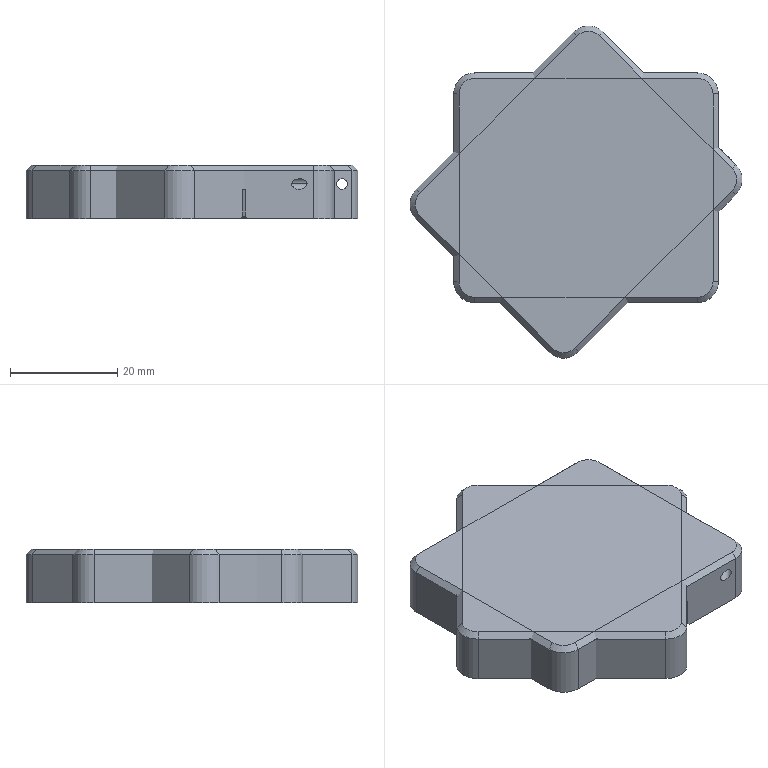NC program | NX | posted with a generic post | part box 61.954 x 61.954 x 10 mm
Whole program:
N10 G17 G21 G94 G90
(ADAPTIVE_MILLING_1 , TOOL : D12开粗)
N12 T02 M6
N14 G54
N16 G17 G0 G90 X-47.087 Y-3.5 B0. C0. S5500 M3
N18 G43 Z30. H2
N20 Z3.1
N22 G94 G1 X-46.937 Y-3.498 Z2.163 F3000.
N24 X-46.787 Y-3.495 Z1.792
N26 X-46.637 Y-3.493 Z1.52
N28 X-46.487 Y-3.491 Z1.3
N30 X-46.337 Y-3.489 Z1.116
N32 X-46.187 Y-3.486 Z0.958
N34 X-46.037 Y-3.484 Z0.82
N36 X-45.887 Y-3.482 Z0.7
N38 X-45.737 Y-3.48 Z0.595
N40 X-45.587 Y-3.477 Z0.502
N42 X-45.437 Y-3.475 Z0.421
N44 X-45.287 Y-3.473 Z0.35
N46 X-45.137 Y-3.471 Z0.29
N48 X-44.987 Y-3.468 Z0.238
N50 X-44.837 Y-3.466 Z0.195
N52 X-44.687 Y-3.464 Z0.161
N54 X-44.537 Y-3.461 Z0.134
N56 X-44.387 Y-3.459 Z0.115
N58 X-44.237 Y-3.457 Z0.104
N60 X-44.087 Y-3.455 Z0.1
N62 X-42.192 Y-3.426
N64 G3 X-41.079 Y-2.649 R1.212
N66 X-40.463 Y0.387 R10.505
N68 X-40.211 Y9.098 R113.687
N70 G1 X-40.2 Y15.678
N72 G2 X-40.18 Y25.077 R512.012
N74 X-37.742 Y29.525 R6.753
N76 X-32.923 Y31.847 R11.427
N78 X-26.975 Y32.564 R31.338
N80 X-14.377 Y32.697 R338.946
N82 G1 X32.076 Y32.698
N84 G2 X36.615 Y30.681 R6.437
N86 X39.166 Y26.099 R10.567
N88 X40.03 Y20.175 R26.789
N90 X40.197 Y9.077 R234.041
N92 G1 X40.199 Y4.677
N94 X40.198 Y-24.619
N96 G2 X38.149 Y-29.145 R6.461
N98 X33.459 Y-31.704 R10.679
N100 X27.429 Y-32.542 R27.958
N102 X16.631 Y-32.696 R246.645
N104 G1 X12.231 Y-32.698
N106 X-32.12 Y-32.697
N108 G2 X-36.646 Y-30.648 R6.462
N110 X-39.205 Y-25.958 R10.681
N112 X-40.042 Y-19.928 R27.995
N114 X-40.196 Y-9.63 R235.867
N116 X-40.144 Y-4.832 R77.851
N118 G3 X-39.603 Y1.94 R216.935
N120 X-39.403 Y14.082 R271.781
N122 G2 X-39.382 Y22.177 R675.391
N124 X-35.797 Y28.613 R8.725
N126 X-30.23 Y31.026 R14.206
N128 X-23.379 Y31.77 R39.402
N130 X-8.58 Y31.898 R456.141
N132 G1 X29.375 Y31.894
N134 G2 X36.05 Y28.379 R8.688
N136 X38.481 Y22.929 R13.975
N138 X39.258 Y16.183 R37.505
N140 X39.397 Y3.784 R341.277
N142 G1 X39.399 Y-21.673
N144 G2 X35.879 Y-28.547 R8.684
N146 X30.331 Y-31.002 R14.053
N148 X23.383 Y-31.769 R38.852
N150 X8.684 Y-31.898 R449.577
N152 G1 X-29.374 Y-31.894
N154 G2 X-36.048 Y-28.378 R8.693
N156 X-38.503 Y-22.828 R14.057
N158 X-39.27 Y-15.88 R38.87
N160 X-39.332 Y-6.182 R142.573
N162 G1 X-38.853 Y1.436
N164 G3 X-38.603 Y15.882 R310.927
N166 G2 X-38.55 Y20.277 R69.413
N168 X-33.953 Y27.909 R10.066
N170 X-27.936 Y30.252 R16.526
N172 X-20.479 Y30.979 R47.05
N174 X-4.98 Y31.097 R535.572
N176 G1 X26.676 Y31.095
N178 G2 X35.514 Y26.29 R10.159
N180 X37.751 Y20.441 R16.681
N182 X38.476 Y13.085 R46.537
N184 X38.598 Y-1.914 R501.258
N186 G1 X38.596 Y-19.214
N188 G2 X33.768 Y-28.028 R10.153
N190 X27.712 Y-30.295 R16.914
N192 X19.952 Y-30.995 R50.455
N194 X4.952 Y-31.097 R603.511
N196 G1 X-26.648 Y-31.095
N198 G2 X-35.516 Y-26.283 R10.16
N200 X-37.795 Y-20.212 R16.896
N202 X-38.486 Y-12.752 R49.142
N204 X-38.238 Y-1.822 R104.868
N206 G3 X-37.806 Y15.587 R293.259
N208 G2 X-37.576 Y19.674 R22.707
N210 X-32.426 Y27.107 R11.028
N212 X-26.079 Y29.448 R18.166
N214 X-18.02 Y30.185 R52.988
N216 X-3.321 Y30.297 R554.733
N218 G1 X24.176 Y30.296
N220 G2 X29.09 Y29.547 R13.62
N222 X34.915 Y24.413 R11.35
N224 X37.037 Y18.092 R19.251
N226 X37.706 Y9.826 R58.88
N228 X37.798 Y-4.474 R658.765
N230 G1 X37.797 Y-16.673
N232 G2 X37.048 Y-21.588 R13.63
N234 X31.911 Y-27.415 R11.354
N236 X25.587 Y-29.536 R19.254
N238 X17.321 Y-30.205 R59.081
N240 X2.722 Y-30.297 R679.393
N242 G1 X-24.374 Y-30.295
N244 G2 X-29.46 Y-29.398 R12.958
N246 X-35.108 Y-24.06 R11.555
N248 X-37.117 Y-17.592 R20.289
N250 X-37.639 Y-6.819 R60.735
N252 X-37.245 Y2.173 R815.993
N254 G3 X-36.996 Y15.605 R483.083
N256 G2 X-35.771 Y21.228 R13.51
N258 X-30.172 Y26.781 R12.359
N260 X-23.494 Y28.798 R21.693
N262 X-14.822 Y29.416 R68.888
N264 X-0.423 Y29.496 R791.053
N266 G1 X22.175 Y29.495
N268 G2 X27.024 Y28.921 R16.905
N270 X33.89 Y23.379 R11.863
N272 X36.148 Y16.887 R19.749
N274 X36.888 Y8.427 R57.67
N276 X36.997 Y-6.572 R593.977
N278 X36.968 Y-15.973 R491.337
N280 X35.306 Y-22.082 R12.637
N282 X29.546 Y-27.084 R12.801
N284 X22.803 Y-28.895 R23.527
N286 X13.724 Y-29.437 R80.469
N288 X0.524 Y-29.496 R796.232
N290 G1 X-22.174 Y-29.495
N292 G2 X-27.022 Y-28.92 R16.896
N294 X-33.889 Y-23.375 R11.869
N296 X-36.129 Y-16.98 R19.668
N298 X-36.788 Y-7.517 R49.35
N300 X-36.414 Y3.241 R588.04
N302 G3 X-36.194 Y14.226 R985.921
N304 G2 X-34.978 Y19.858 R14.612
N306 X-29.08 Y25.845 R12.846
N308 X-22.127 Y27.962 R22.483
N310 X-13.057 Y28.613 R71.08
N312 X1.843 Y28.696 R805.214
N314 G1 X20.176 Y28.695
N316 G2 X25.142 Y28.232 R21.058
N318 X32.876 Y22.413 R12.364
N320 X35.285 Y15.664 R20.243
N322 X36.074 Y7.008 R57.951
N324 X36.196 Y-8.391 R556.749
N326 X36.14 Y-14.773 R145.792
N328 X34.231 Y-21.221 R13.268
N330 X28.224 Y-26.257 R13.497
N332 X21.186 Y-28.094 R24.935
N334 X12.006 Y-28.634 R84.46
N336 X-1.194 Y-28.696 R789.14
N338 G1 X-20.194 Y-28.694
N340 G2 X-25.159 Y-28.226 R20.841
N342 X-32.953 Y-22.279 R12.39
N344 X-35.304 Y-15.514 R20.401
N346 X-35.907 Y-6.747 R48.303
N348 X-35.566 Y5.105 R774.796
N350 X-35.388 Y13.046 R564.731
N352 X-34.008 Y18.946 R15.215
N354 X-27.932 Y24.979 R13.372
N356 X-20.98 Y27.108 R23.087
N358 X-12.313 Y27.788 R67.73
N360 X2.586 Y27.895 R629.437
N362 G1 X18.386 Y27.894
N364 G2 X23.559 Y27.471 R24.709
N366 X32.07 Y21.168 R12.879
N368 X34.447 Y14.4 R21.12
N370 X35.263 Y5.646 R58.782
N372 X35.359 Y-12.752 R477.337
N374 X34.193 Y-18.5 R15.721
N376 X28.182 Y-24.841 R13.195
N378 X21.148 Y-27.078 R22.584
N380 X12.483 Y-27.782 R65.83
N382 X-3.516 Y-27.895 R642.924
N384 G1 X-18.274 Y-27.894
N386 G2 X-23.449 Y-27.493 R25.544
N388 X-32.068 Y-21.165 R12.877
N390 X-34.476 Y-14.09 R20.871
N392 X-35.029 Y-5.619 R50.258
N394 X-34.752 Y5.89 R768.444
N396 X-34.567 Y12.167 R144.064
N398 X-32.826 Y18.484 R15.184
N400 X-26.471 Y24.296 R14.08
N402 X-19.385 Y26.337 R24.783
N404 X-9.915 Y27.007 R76.762
N406 X4.484 Y27.095 R780.18
N408 G1 X16.876 Y27.092
N410 G2 X22.249 Y26.663 R26.883
N412 X31.171 Y20.134 R13.309
N414 X33.634 Y13.085 R21.832
N416 X34.459 Y4.132 R61.158
N418 X34.554 Y-11.267 R352.152
N420 X33.479 Y-17.038 R17.132
N422 X27.197 Y-23.916 R13.523
N424 X20.09 Y-26.22 R22.917
N426 X11.129 Y-26.974 R65.955
N428 X-4.57 Y-27.095 R601.629
N430 G1 X-16.57 Y-27.094
N432 G2 X-21.949 Y-26.721 R29.489
N434 X-31.269 Y-19.954 R13.341
N436 X-33.631 Y-12.771 R21.45
N438 X-34.159 Y-4.297 R53.449
N440 X-33.827 Y10.181 R613.148
N442 X-32.604 Y16.126 R17.909
N444 X-26.094 Y23.091 R14.015
N446 X-18.886 Y25.402 R23.656
N448 X-9.925 Y26.164 R66.715
N450 X6.574 Y26.295 R603.817
N452 X17.273 Y26.255 R504.016
N454 X23.066 Y25.276 R18.786
N456 X30.475 Y18.785 R13.831
N458 X32.862 Y11.605 R23.098
N460 X33.661 Y2.548 R64.779
N462 X33.74 Y-10.05 R239.906
N464 X32.642 Y-15.919 R17.856
N466 X26.098 Y-23.074 R13.914
N468 X18.987 Y-25.38 R23.444
N470 X9.829 Y-26.166 R66.354
N472 X-6.27 Y-26.294 R597.162
N474 X-17.174 Y-26.258 R495.505
N476 X-22.878 Y-25.341 R19.251
N478 X-30.457 Y-18.789 R13.736
N480 X-32.752 Y-11.68 R21.853
N482 X-33.297 Y-3.106 R55.449
N484 X-33.039 Y8.983 R305.003
N486 X-31.792 Y15.027 R18.742
N488 X-25.173 Y22.181 R14.328
N490 X-17.978 Y24.537 R23.837
N492 X-8.722 Y25.356 R66.184
N494 X8.077 Y25.494 R588.727
N496 X16.575 Y25.423 R209.725
N498 X22.62 Y24.194 R17.974
N500 X29.679 Y17.644 R14.244
N502 X32.04 Y10.447 R23.786
N504 X32.851 Y1.391 R65.28
N506 X32.916 Y-9.007 R159.97
N508 X31.678 Y-15.151 R17.919
N510 X25.19 Y-22.151 R14.244
N512 X17.996 Y-24.528 R23.665
N514 X8.741 Y-25.354 R65.627
N516 X-8.458 Y-25.494 R598.535
N518 X-16.656 Y-25.417 R186.832
N520 X-22.787 Y-24.121 R17.683
N522 X-29.797 Y-17.358 R14.191
N524 X-31.968 Y-10. R23.332
N526 X-32.444 Y-1.02 R64.421
N528 X-32.217 Y8.275 R151.413
N530 X-30.718 Y14.564 R18.12
N532 X-23.961 Y21.44 R14.781
N534 X-16.547 Y23.771 R24.934
N536 X-7.187 Y24.56 R70.271
N538 X14.412 Y24.655 R644.798
N540 X20.236 Y23.836 R22.251
N542 X28.703 Y16.862 R14.396
N544 X31.152 Y9.695 R23.603
N546 X32.038 Y0.345 R63.647
N548 X32.076 Y-8.153 R104.784
N550 X30.683 Y-14.464 R17.671
N552 X24.029 Y-21.379 R14.587
N554 X16.632 Y-23.75 R24.626
N556 X7.474 Y-24.549 R68.103
N558 X-9.824 Y-24.694 R591.965
N560 X-16.42 Y-24.539 R79.28
N562 X-23.184 Y-22.567 R16.171
N564 X-29.199 Y-15.781 R14.816
N566 X-31.199 Y-8.17 R25.383
N568 X-31.597 Y1.115 R76.181
N570 X-31.327 Y8.107 R68.591
N572 X-29.12 Y15.002 R16.536
N574 X-22.425 Y20.868 R15.514
N576 X-14.961 Y23.033 R26.857
N578 X-5.395 Y23.773 R77.026
N580 X13.403 Y23.844 R484.321
N582 X19.416 Y22.938 R22.243
N584 X27.784 Y15.998 R14.649
N586 X30.343 Y8.546 R23.972
N588 X31.223 Y-0.603 R63.698
N590 X31.173 Y-7.998 R61.479
N592 X29.024 Y-15.012 R16.112
N594 X22.44 Y-20.832 R15.346
N596 X14.78 Y-23.054 R26.829
N598 X5.513 Y-23.768 R76.96
N600 X-13.286 Y-23.847 R498.573
N602 X-19.304 Y-22.971 R22.656
N604 X-27.851 Y-15.751 R14.455
N606 X-30.182 Y-8.241 R23.424
N608 X-30.754 Y1.033 R64.446
N610 X-30.418 Y7.819 R47.863
N612 X-27.144 Y15.654 R15.701
N614 X-20.173 Y20.583 R16.838
N616 X-12.404 Y22.425 R31.622
N618 X-2.026 Y23.02 R102.326
N620 X12.073 Y23.044 R402.694
N622 X18.289 Y22.145 R23.455
N624 X26.968 Y14.975 R14.921
N626 X29.5 Y7.612 R24.319
N628 X30.424 Y-2.235 R63.43
N630 X30.098 Y-8.716 R33.378
N632 X22.511 Y-19.438 R14.847
N634 X15.064 Y-22.004 R24.247
N636 X5.617 Y-22.921 R64.543
N638 X-12.08 Y-23.043 R382.648
N640 X-18.104 Y-22.198 R23.668
N642 X-27.036 Y-14.675 R14.682
N644 X-29.316 Y-7.248 R23.973
N646 X-29.723 Y5.719 R59.734
N648 X-27.637 Y12.761 R17.448
N650 X-20.718 Y19.078 R15.811
N652 X-12.983 Y21.379 R27.22
N654 X-3.321 Y22.157 R76.946
N656 X11.278 Y22.224 R281.36
N658 X17.483 Y21.257 R22.963
N660 X26.132 Y14.007 R15.16
N662 X28.684 Y6.564 R24.744
N664 X29.49 Y-5.583 R52.906
N666 X27.553 Y-12.668 R16.907
N668 X20.753 Y-19.018 R15.545
N670 X13.32 Y-21.312 R26.419
N672 X3.562 Y-22.148 R72.859
N674 X-11.336 Y-22.222 R276.001
N676 X-17.632 Y-21.203 R22.555
N678 X-26.136 Y-13.777 R14.883
N680 X-28.456 Y-6.254 R24.259
N682 X-28.847 Y5.013 R47.774
N684 X-26.465 Y12.374 R16.949
N686 X-19.499 Y18.372 R16.218
N688 X-11.735 Y20.6 R28.291
N690 X-1.97 Y21.361 R80.32
N692 X10.328 Y21.409 R211.35
N694 X16.72 Y20.359 R22.889
N696 X25.336 Y12.982 R15.405
N698 X27.905 Y5.336 R25.378
N700 X28.579 Y-4.917 R42.719
N702 X26.235 Y-12.493 R16.284
N704 X19.541 Y-18.303 R15.96
N706 X11.881 Y-20.564 R27.576
N708 X2.02 Y-21.357 R77.747
N710 X-10.378 Y-21.406 R207.67
N712 X-16.576 Y-20.399 R22.758
N714 X-25.247 Y-12.876 R15.038
N716 X-27.601 Y-5.264 R24.573
N718 X-27.938 Y4.405 R38.333
N720 X-25.047 Y12.297 R16.335
N722 X-18.032 Y17.777 R16.826
N724 X-10.127 Y19.874 R30.253
N726 X0.243 Y20.587 R90.867
N728 X9.94 Y20.562 R132.849
N730 X16.488 Y19.265 R21.092
N732 X24.554 Y11.947 R15.64
N734 X27.096 Y4.279 R25.737
N736 X27.623 Y-4.482 R34.143
N738 X24.505 Y-12.792 R15.538
N740 X17.664 Y-17.887 R16.874
N742 X9.739 Y-19.917 R30.909
N744 X-0.334 Y-20.587 R93.156
N746 X-9.732 Y-20.573 R137.837
N748 X-16.193 Y-19.363 R21.519
N750 X-24.319 Y-12.062 R15.191
N752 X-26.75 Y-4.243 R24.619
N754 X-26.917 Y4.426 R30.072
N756 X-18.905 Y16.044 R15.566
N758 X-11.286 Y18.699 R25.3
N760 X-1.644 Y19.688 R65.027
N762 X8.952 Y19.742 R119.084
N764 X15.499 Y18.455 R21.447
N766 X23.686 Y11.085 R15.801
N768 X26.295 Y3.121 R25.587
N770 X26.561 Y-4.646 R26.347
N772 X19.195 Y-15.789 R15.063
N774 X11.627 Y-18.609 R24.089
N776 X2.195 Y-19.659 R60.494
N778 X-8.901 Y-19.744 R121.022
N780 X-15.353 Y-18.489 R21.289
N782 X-23.47 Y-11.112 R15.361
N784 X-25.952 Y-2.716 R24.58
N786 X-25.753 Y4.847 R22.965
N788 X-18.365 Y14.985 R15.375
N790 X-10.799 Y17.785 R24.533
N792 X-1.369 Y18.848 R60.637
N794 X8.127 Y18.907 R94.394
N796 X14.76 Y17.549 R21.147
N798 X22.88 Y10.117 R15.979
N800 X25.641 Y-3.237 R25.057
N802 X18.527 Y-14.78 R14.926
N804 X11.103 Y-17.692 R23.421
N806 X1.982 Y-18.811 R56.275
N808 X-8.213 Y-18.899 R93.99
N810 X-14.833 Y-17.488 R20.438
N812 X-22.685 Y-10.049 R15.541
N814 X-24.989 Y2.773 R23.106
N816 X-17.732 Y13.97 R15.182
N818 X-10.094 Y16.914 R24.077
N820 X-0.77 Y18.02 R58.276
N822 X8.024 Y18.01 R67.843
N824 X15.224 Y16.082 R19.027
N826 X22.199 Y8.916 R16.28
N828 X24.606 Y-2.41 R22.033
N830 X17.937 Y-13.708 R14.637
N832 X10.489 Y-16.791 R22.709
N834 X1.378 Y-17.981 R53.602
N836 X-7.716 Y-18.032 R71.62
N838 X-14.665 Y-16.31 R19.238
N840 X-21.971 Y-8.841 R15.777
N842 X-23.907 Y2.34 R20.17
N844 X-17.258 Y12.836 R14.821
N846 X-9.708 Y15.967 R23.033
N848 X-0.196 Y17.186 R54.24
N850 X7.795 Y17.1 R51.495
N852 X15.358 Y14.658 R17.868
N854 X21.78 Y7.135 R16.747
N856 X23.466 Y-2.213 R18.908
N858 X17.21 Y-12.71 R14.283
N860 X9.787 Y-15.907 R22.204
N862 X0.485 Y-17.163 R51.685
N864 X-7.607 Y-17.112 R52.21
N866 X-14.989 Y-14.799 R17.649
N868 X-21.549 Y-6.915 R16.172
N870 X-22.676 Y2.495 R17.225
N872 X-16.587 Y11.808 R14.432
N874 X-9.093 Y15.067 R22.342
N876 X1.006 Y16.371 R51.385
N878 X8.287 Y16.056 R35.918
N880 X17.55 Y11.327 R16.237
N882 X22.341 Y-0.948 R17.277
N884 X16.775 Y-11.472 R13.779
N886 X9.568 Y-14.89 R20.879
N888 X0.188 Y-16.301 R46.381
N890 X-7.399 Y-16.174 R41.017
N892 X-15.259 Y-13.167 R16.614
N894 X-21.643 Y0.8 R16.019
N896 X-16.174 Y10.554 R13.807
N898 X-8.917 Y14.041 R20.936
N900 X1.657 Y15.506 R45.33
N902 X8.812 Y14.91 R27.575
N904 X21.084 Y0.398 R15.761
N906 X16.283 Y-10.204 R13.121
N908 X9.32 Y-13.853 R19.54
N910 X-0.028 Y-15.42 R41.101
N912 X-7.408 Y-15.17 R32.551
N914 X-16.388 Y-10.516 R15.634
N916 X-20.403 Y-0.317 R14.513
N918 X-15.838 Y9.148 R13.063
N920 X-8.848 Y12.948 R19.301
N922 X5.288 Y14.469 R38.155
N924 X13.502 Y11.591 R17.106
N926 X19.596 Y2.157 R14.54
N928 X15.943 Y-8.694 R12.346
N930 X9.292 Y-12.705 R17.893
N932 X-0.213 Y-14.512 R35.594
N934 X-7.478 Y-14.102 R26.727
N936 X-16.815 Y-7.952 R14.837
N938 X-18.617 Y2.181 R12.319
N940 X-13.63 Y9.236 R13.195
N942 X-6.49 Y12.524 R20.829
N944 X4.809 Y13.516 R32.596
N946 X13.043 Y10.418 R16.394
N948 X18.071 Y2.79 R13.119
N950 X15.217 Y-7.407 R11.552
N952 X8.903 Y-11.63 R16.604
N954 X-4.854 Y-13.48 R30.739
N956 X-12.781 Y-10.398 R15.603
N958 X-17.429 Y-2.682 R12.062
N960 X-14.51 Y6.549 R11.391
N962 X-8.164 Y10.81 R16.515
N964 X4.506 Y12.511 R27.349
N966 X12.619 Y9.149 R15.357
N968 X16.684 Y2.002 R11.312
N970 X13.933 Y-6.611 R10.934
N972 X7.732 Y-10.827 R15.977
N974 X-4.34 Y-12.486 R25.982
N976 X-11.863 Y-9.477 R14.638
N978 X-15.922 Y-1.616 R10.516
N980 X-12.808 Y6.181 R10.942
N982 X-6.422 Y10.213 R16.339
N984 X4.405 Y11.434 R22.874
N986 X11.628 Y8.257 R13.95
N988 X13.47 Y-4.529 R9.762
N990 X7.944 Y-9.358 R13.687
N992 X-4.212 Y-11.392 R21.394
N994 X-10.677 Y-8.677 R13.048
N996 X-12.99 Y3.078 R9.329
N998 X-7.764 Y8.206 R12.83
N1000 X4.435 Y10.266 R18.922
N1002 X10.399 Y7.415 R11.842
N1004 X12.299 Y-2.886 R8.812
N1006 X7.406 Y-8.067 R12.006
N1008 X-4.264 Y-10.18 R17.347
N1010 X-9.662 Y-7.519 R10.456
N1012 X-11.488 Y1.737 R8.396
N1014 X-6.723 Y7.113 R11.415
N1016 X4.169 Y9.039 R15.315
N1018 X9.218 Y6.172 R9.05
N1020 X10.413 Y-2.016 R7.979
N1022 X5.786 Y-7.213 R10.838
N1024 X-3.453 Y-8.971 R13.64
N1026 X-8.623 Y-5.684 R7.748
N1028 X-9.11 Y1.593 R7.676
N1030 X-3.895 Y6.772 R10.443
N1032 X2.832 Y7.781 R11.31
N1034 X8.3 Y0.161 R6.675
N1036 X4.559 Y-5.707 R8.729
N1038 X-0.97 Y-7.493 R9.402
N1040 X-6.536 Y-2.008 R5.733
N1042 X-2.166 Y5.022 R7.29
N1044 X1.019 Y4.782 R3.77
N1046 X3.153 Y3.006 R6.297
N1048 G1 X3.246 Y2.888 Z0.104
N1050 X3.34 Y2.771 Z0.115
N1052 X3.433 Y2.654 Z0.134
N1054 X3.527 Y2.537 Z0.161
N1056 X3.62 Y2.419 Z0.195
N1058 X3.714 Y2.302 Z0.238
N1060 X3.807 Y2.185 Z0.29
N1062 X3.901 Y2.068 Z0.35
N1064 X3.994 Y1.95 Z0.421
N1066 X4.088 Y1.833 Z0.502
N1068 X4.181 Y1.716 Z0.595
N1070 X4.275 Y1.598 Z0.7
N1072 X4.368 Y1.481 Z0.82
N1074 X4.462 Y1.364 Z0.958
N1076 X4.556 Y1.247 Z1.116
N1078 X4.649 Y1.129 Z1.3
N1080 X4.743 Y1.012 Z1.52
N1082 X4.836 Y0.895 Z1.792
N1084 X4.93 Y0.778 Z2.163
N1086 X5.023 Y0.66 Z3.1
N1088 G0 Z30.
N1090 M5
(一刀光面_COPY , TOOL : D50面刀)
N1092 T01 M6
N1094 G54
N1096 G17 G0 G90 X60.18 Y0. B0. C0. S3500 M3
N1098 G43 Z30. H1
N1100 Z2.
N1102 G94 G1 Z0. F800.
N1104 X55.18
N1106 X-55.18
N1108 X-60.18
N1110 Z2.
N1112 G0 Z30.
N1114 M5
(PLANAR_MILL_3_COPY_COPY_COPY , TOOL : D8倒角刀)
N1116 T05 M6
N1118 G54
N1120 G17 G0 G90 X-27.88 Y-2. B0. C0. S3500 M3
N1122 G43 Z30. H5
N1124 Z0.
N1126 G94 G1 Z-2. F800.
N1128 G3 X-25.88 Y0. R2.
N1130 G1 Y17.5
N1132 G2 X-20.75 Y22.63 R5.13
N1134 G1 X20.75
N1136 G2 X25.88 Y17.5 R5.13
N1138 G1 Y-17.5
N1140 G2 X20.75 Y-22.63 R5.13
N1142 G1 X-20.75
N1144 G2 X-25.88 Y-17.5 R5.13
N1146 G1 Y0.
N1148 G3 X-27.88 Y2. R2.
N1150 G1 Z0.
N1152 G0 Z30.
N1154 M5
N1156 M2